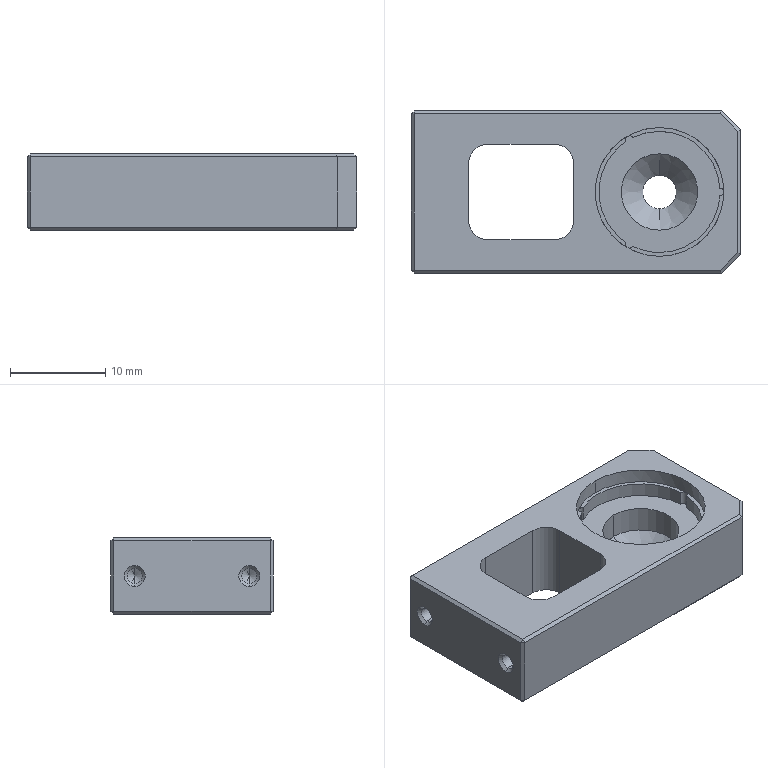NC program | NX | posted with a generic post | part box 34.5 x 17 x 8 mm
Lines 3981 to 4112 of 4112:
(PLANAR_MILL_COPY_1 , TOOL : D6A45)
N7906 T07 M6
N7908 G54
N7910 G17 G0 G90 X15.695 Y10.325 S9500 M3
N7912 G43 Z30. H7
N7914 Z0.5
N7916 G94 G1 Z-1. F1250.
N7918 X15.574 Y9.873
N7920 G3 X15.833 Y8.907 R1.
N7922 G1 X17.657 Y7.083
N7924 G2 X17.95 Y6.376 R1.
N7926 G1 Y-6.376
N7928 G2 X17.657 Y-7.083 R1.
N7930 G1 X15.833 Y-8.907
N7932 G2 X15.126 Y-9.2 R1.
N7934 G1 X-16.95
N7936 G2 X-17.95 Y-8.2 R1.
N7938 G1 Y8.2
N7940 G2 X-16.95 Y9.2 R1.
N7942 G1 X15.126
N7944 G2 X15.833 Y8.907 R1.
N7946 G3 X16.799 Y8.648 R1.
N7948 G1 X17.58 Y8.857
N7950 Z0.5
N7952 G0 Z30.
(PLANAR_MILL_COPY_1_COPY , TOOL : D6A45)
N7954 X10.144 Y4.436
N7956 Z0.5
N7958 G1 Z-1.
N7960 X9.616 Y5.35
N7962 G3 X8.75 Y5.85 R1.
N7964 X2.9 Y0. R5.85
N7966 X8.75 Y5.85 R-5.85
N7968 X7.884 Y5.35 R1.
N7970 G1 X7.356 Y4.436
N7972 Z0.5
N7974 G0 Z30.
N7976 X-2.35 Y1.73
N7978 Z0.5
N7980 G1 Z-1.
N7982 X-1.65 Y2.134
N7984 G3 X-1.15 Y3. R1.
N7986 X-2.25 Y4.1 R1.1
N7988 G1 X-9.25
N7990 G3 X-10.35 Y3. R1.1
N7992 G1 Y-3.
N7994 G3 X-9.25 Y-4.1 R1.1
N7996 G1 X-2.25
N7998 G3 X-1.15 Y-3. R1.1
N8000 G1 Y3.
N8002 G3 X-1.65 Y3.866 R1.
N8004 G1 X-2.35 Y2.9
N8006 Z0.5
N8008 G0 Z30.
N8010 M5
(DRILLING , TOOL : D1)
N8012 T01 M6
N8014 G54
N8016 G17 G0 G90 X5.675 Y5.326 S4000 M3
N8018 G43 Z30. H1
N8020 G94 G83 G99 Z-3. F70. Q0.5 R1.5
N8022 Y-5.326
N8024 X14.9 Y0.
N8026 G80
N8028 G0 X14.9 Y0. Z30.
N8030 M5
(刀补4 , TOOL : D4)
N8032 T04 M6
N8034 G54
N8036 G17 G0 G90 X6.134 Y-2.197 S9500 M3
N8038 G43 Z30. H4
N8040 Z-1.5
N8042 G94 G1 Z-3. F1000.
N8044 G41 X6.105 Y-2.293 D4
N8046 X6.014 Y-3.061
N8048 G3 X6.171 Y-3.429 R0.4
N8050 G1 X6.334 Y-3.551 F1200.
N8052 X6.587 Y-3.725
N8054 G3 X6.853 Y-3.859 R41.289
N8056 X13.048 Y-0.122 R4.3
N8058 X13.022 Y0.406 R3.377
N8060 G1 X13.03 Y0.417
N8062 G3 X7.09 Y3.967 R4.3
N8064 G1 X7.076 Y3.95
N8066 G3 X6.492 Y3.662 R3.013
N8068 G1 X6.37 Y3.581
N8070 G3 X6.157 Y-3.43 R4.3
N8072 G1 X6.171 Y-3.429
N8074 G3 X6.501 Y-3.202 R0.4
N8076 G1 X6.686 Y-2.815
N8078 G40
N8080 X6.713 Y-2.719
N8082 Z-1.5
N8084 G0 Z30.
(111 , TOOL : D4)
N8086 X-18.217 Y12.294
N8088 Z-5.85
N8090 G1 Z-7.85 F1000.
N8092 X-17.296 Y10.7
N8094 G3 X-16.95 Y10.5 R0.4
N8096 G1 X15.25 F1200.
N8098 G2 X16.664 Y9.914 R2.
N8100 G1 X18.664 Y7.914
N8102 G2 X19.25 Y6.5 R2.
N8104 G1 Y-6.5
N8106 G2 X18.664 Y-7.914 R2.
N8108 G1 X16.664 Y-9.914
N8110 G2 X15.25 Y-10.5 R2.
N8112 G1 X-16.95
N8114 G2 X-18.364 Y-9.914 R2.
N8116 G1 X-18.664 Y-9.614
N8118 G2 X-19.25 Y-8.2 R2.
N8120 G1 Y8.2
N8122 G2 X-18.664 Y9.614 R2.
N8124 G1 X-18.364 Y9.914
N8126 G2 X-16.95 Y10.5 R2.
N8128 G3 X-16.604 Y10.7 R0.4
N8130 G1 X-15.564 Y12.5
N8132 Z-5.85
N8134 G0 Z30.
N8136 M5
N8138 M2